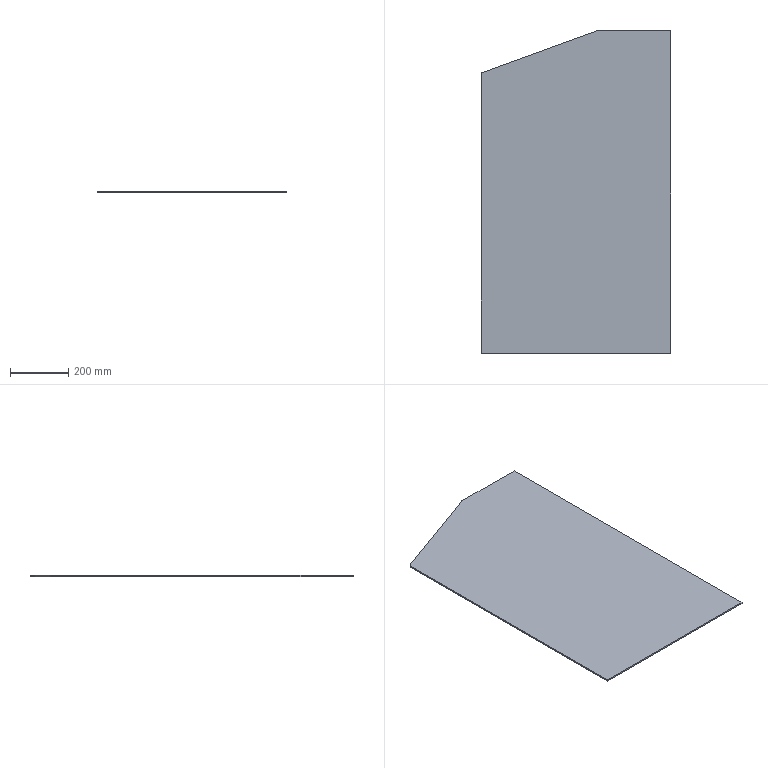Part | SolidWorks | features Extrusion 1, Fillet 1 | 1 solid | 9 faces | box 651 x 1106 x 5 mm | volume 3454699 mm3 | plane 7 | cylinder 2 | commonest cylinder face diameters 12 x2
STEP:
#1=CARTESIAN_POINT('',(-651.,0.,0.));
#2=VERTEX_POINT('',#1);
#3=CARTESIAN_POINT('',(0.,0.,0.));
#4=VERTEX_POINT('',#3);
#5=CARTESIAN_POINT('',(-651.,0.,0.));
#6=DIRECTION('',(1.,0.,0.));
#7=VECTOR('',#6,1000.);
#8=LINE('',#5,#7);
#9=EDGE_CURVE('',#2,#4,#8,.T.);
#10=ORIENTED_EDGE('',*,*,#9,.T.);
#11=CARTESIAN_POINT('',(0.,0.,5.));
#12=VERTEX_POINT('',#11);
#13=CARTESIAN_POINT('',(0.,0.,5.));
#14=DIRECTION('',(0.,0.,-1.));
#15=VECTOR('',#14,1000.);
#16=LINE('',#13,#15);
#17=EDGE_CURVE('',#12,#4,#16,.T.);
#18=ORIENTED_EDGE('',*,*,#17,.F.);
#19=CARTESIAN_POINT('',(-651.,0.,5.));
#20=VERTEX_POINT('',#19);
#21=CARTESIAN_POINT('',(-651.,0.,5.));
#22=DIRECTION('',(1.,0.,0.));
#23=VECTOR('',#22,1000.);
#24=LINE('',#21,#23);
#25=EDGE_CURVE('',#20,#12,#24,.T.);
#26=ORIENTED_EDGE('',*,*,#25,.F.);
#27=CARTESIAN_POINT('',(-651.,0.,5.));
#28=DIRECTION('',(0.,0.,-1.));
#29=VECTOR('',#28,1000.);
#30=LINE('',#27,#29);
#31=EDGE_CURVE('',#20,#2,#30,.T.);
#32=ORIENTED_EDGE('',*,*,#31,.T.);
#33=EDGE_LOOP('',(#10,#18,#26,#32));
#34=FACE_OUTER_BOUND('',#33,.T.);
#35=CARTESIAN_POINT('',(-651.,0.,5.));
#36=DIRECTION('',(0.,1.,0.));
#37=DIRECTION('',(0.,0.,1.));
#38=AXIS2_PLACEMENT_3D('',#35,#36,#37);
#39=PLANE('',#38);
#40=ADVANCED_FACE('',(#34),#39,.F.);
#41=CARTESIAN_POINT('',(0.,1105.5,0.));
#42=VERTEX_POINT('',#41);
#43=CARTESIAN_POINT('',(0.,0.,0.));
#44=DIRECTION('',(0.,1.,0.));
#45=VECTOR('',#44,1000.);
#46=LINE('',#43,#45);
#47=EDGE_CURVE('',#4,#42,#46,.T.);
#48=ORIENTED_EDGE('',*,*,#47,.T.);
#49=CARTESIAN_POINT('',(0.,1105.5,5.));
#50=VERTEX_POINT('',#49);
#51=CARTESIAN_POINT('',(0.,1105.5,5.));
#52=DIRECTION('',(0.,0.,-1.));
#53=VECTOR('',#52,1000.);
#54=LINE('',#51,#53);
#55=EDGE_CURVE('',#50,#42,#54,.T.);
#56=ORIENTED_EDGE('',*,*,#55,.F.);
#57=CARTESIAN_POINT('',(0.,0.,5.));
#58=DIRECTION('',(0.,1.,0.));
#59=VECTOR('',#58,1000.);
#60=LINE('',#57,#59);
#61=EDGE_CURVE('',#12,#50,#60,.T.);
#62=ORIENTED_EDGE('',*,*,#61,.F.);
#63=ORIENTED_EDGE('',*,*,#17,.T.);
#64=EDGE_LOOP('',(#48,#56,#62,#63));
#65=FACE_OUTER_BOUND('',#64,.T.);
#66=CARTESIAN_POINT('',(0.,0.,5.));
#67=DIRECTION('',(-1.,0.,0.));
#68=DIRECTION('',(0.,0.,1.));
#69=AXIS2_PLACEMENT_3D('',#66,#67,#68);
#70=PLANE('',#69);
#71=ADVANCED_FACE('',(#65),#70,.F.);
#72=CARTESIAN_POINT('',(-252.562,1105.5,0.));
#73=VERTEX_POINT('',#72);
#74=CARTESIAN_POINT('',(0.,1105.5,0.));
#75=DIRECTION('',(-1.,0.,0.));
#76=VECTOR('',#75,1000.);
#77=LINE('',#74,#76);
#78=EDGE_CURVE('',#42,#73,#77,.T.);
#79=ORIENTED_EDGE('',*,*,#78,.T.);
#80=CARTESIAN_POINT('',(-252.562,1105.5,5.));
#81=VERTEX_POINT('',#80);
#82=CARTESIAN_POINT('',(-252.562,1105.5,5.));
#83=DIRECTION('',(0.,0.,1.));
#84=VECTOR('',#83,1000.);
#85=LINE('',#82,#84);
#86=EDGE_CURVE('',#73,#81,#85,.T.);
#87=ORIENTED_EDGE('',*,*,#86,.T.);
#88=CARTESIAN_POINT('',(0.,1105.5,5.));
#89=DIRECTION('',(-1.,0.,0.));
#90=VECTOR('',#89,1000.);
#91=LINE('',#88,#90);
#92=EDGE_CURVE('',#50,#81,#91,.T.);
#93=ORIENTED_EDGE('',*,*,#92,.F.);
#94=ORIENTED_EDGE('',*,*,#55,.T.);
#95=EDGE_LOOP('',(#79,#87,#93,#94));
#96=FACE_OUTER_BOUND('',#95,.T.);
#97=CARTESIAN_POINT('',(0.,1105.5,5.));
#98=DIRECTION('',(0.,-1.,0.));
#99=DIRECTION('',(0.,0.,-1.));
#100=AXIS2_PLACEMENT_3D('',#97,#98,#99);
#101=PLANE('',#100);
#102=ADVANCED_FACE('',(#96),#101,.F.);
#103=CARTESIAN_POINT('',(-254.614,1105.138,5.));
#104=VERTEX_POINT('',#103);
#105=CARTESIAN_POINT('',(-647.052,962.302,5.));
#106=VERTEX_POINT('',#105);
#107=CARTESIAN_POINT('',(-253.62,1105.5,5.));
#108=DIRECTION('',(-0.9397,-0.342,0.));
#109=VECTOR('',#108,1000.);
#110=LINE('',#107,#109);
#111=EDGE_CURVE('',#104,#106,#110,.T.);
#112=ORIENTED_EDGE('',*,*,#111,.F.);
#113=CARTESIAN_POINT('',(-254.614,1105.138,0.));
#114=VERTEX_POINT('',#113);
#115=CARTESIAN_POINT('',(-254.614,1105.138,5.));
#116=DIRECTION('',(0.,0.,-1.));
#117=VECTOR('',#116,1000.);
#118=LINE('',#115,#117);
#119=EDGE_CURVE('',#104,#114,#118,.T.);
#120=ORIENTED_EDGE('',*,*,#119,.T.);
#121=CARTESIAN_POINT('',(-647.052,962.302,0.));
#122=VERTEX_POINT('',#121);
#123=CARTESIAN_POINT('',(-253.62,1105.5,0.));
#124=DIRECTION('',(-0.9397,-0.342,0.));
#125=VECTOR('',#124,1000.);
#126=LINE('',#123,#125);
#127=EDGE_CURVE('',#114,#122,#126,.T.);
#128=ORIENTED_EDGE('',*,*,#127,.T.);
#129=CARTESIAN_POINT('',(-647.052,962.302,5.));
#130=DIRECTION('',(0.,0.,1.));
#131=VECTOR('',#130,1000.);
#132=LINE('',#129,#131);
#133=EDGE_CURVE('',#122,#106,#132,.T.);
#134=ORIENTED_EDGE('',*,*,#133,.T.);
#135=EDGE_LOOP('',(#112,#120,#128,#134));
#136=FACE_OUTER_BOUND('',#135,.T.);
#137=CARTESIAN_POINT('',(-253.62,1105.5,5.));
#138=DIRECTION('',(0.342,-0.9397,0.));
#139=DIRECTION('',(0.9397,0.342,0.));
#140=AXIS2_PLACEMENT_3D('',#137,#138,#139);
#141=PLANE('',#140);
#142=ADVANCED_FACE('',(#136),#141,.F.);
#143=CARTESIAN_POINT('',(-651.,956.664,5.));
#144=VERTEX_POINT('',#143);
#145=CARTESIAN_POINT('',(-651.,960.866,5.));
#146=DIRECTION('',(0.,-1.,0.));
#147=VECTOR('',#146,1000.);
#148=LINE('',#145,#147);
#149=EDGE_CURVE('',#144,#20,#148,.T.);
#150=ORIENTED_EDGE('',*,*,#149,.F.);
#151=CARTESIAN_POINT('',(-651.,956.664,0.));
#152=VERTEX_POINT('',#151);
#153=CARTESIAN_POINT('',(-651.,956.664,5.));
#154=DIRECTION('',(0.,0.,-1.));
#155=VECTOR('',#154,1000.);
#156=LINE('',#153,#155);
#157=EDGE_CURVE('',#144,#152,#156,.T.);
#158=ORIENTED_EDGE('',*,*,#157,.T.);
#159=CARTESIAN_POINT('',(-651.,960.866,0.));
#160=DIRECTION('',(0.,-1.,0.));
#161=VECTOR('',#160,1000.);
#162=LINE('',#159,#161);
#163=EDGE_CURVE('',#152,#2,#162,.T.);
#164=ORIENTED_EDGE('',*,*,#163,.T.);
#165=ORIENTED_EDGE('',*,*,#31,.F.);
#166=EDGE_LOOP('',(#150,#158,#164,#165));
#167=FACE_OUTER_BOUND('',#166,.T.);
#168=CARTESIAN_POINT('',(-651.,960.866,5.));
#169=DIRECTION('',(1.,0.,0.));
#170=DIRECTION('',(0.,1.,0.));
#171=AXIS2_PLACEMENT_3D('',#168,#169,#170);
#172=PLANE('',#171);
#173=ADVANCED_FACE('',(#167),#172,.F.);
#174=ORIENTED_EDGE('',*,*,#92,.T.);
#175=CARTESIAN_POINT('',(-252.562,1099.5,5.));
#176=DIRECTION('',(0.,0.,1.));
#177=DIRECTION('',(1.,0.,0.));
#178=AXIS2_PLACEMENT_3D('',#175,#176,#177);
#179=CIRCLE('',#178,6.);
#180=EDGE_CURVE('',#81,#104,#179,.T.);
#181=ORIENTED_EDGE('',*,*,#180,.T.);
#182=ORIENTED_EDGE('',*,*,#111,.T.);
#183=CARTESIAN_POINT('',(-645.,956.664,5.));
#184=DIRECTION('',(0.,0.,1.));
#185=DIRECTION('',(1.,0.,0.));
#186=AXIS2_PLACEMENT_3D('',#183,#184,#185);
#187=CIRCLE('',#186,6.);
#188=EDGE_CURVE('',#106,#144,#187,.T.);
#189=ORIENTED_EDGE('',*,*,#188,.T.);
#190=ORIENTED_EDGE('',*,*,#149,.T.);
#191=ORIENTED_EDGE('',*,*,#25,.T.);
#192=ORIENTED_EDGE('',*,*,#61,.T.);
#193=EDGE_LOOP('',(#174,#181,#182,#189,#190,#191,#192));
#194=FACE_OUTER_BOUND('',#193,.T.);
#195=CARTESIAN_POINT('',(0.,0.,5.));
#196=DIRECTION('',(0.,0.,1.));
#197=DIRECTION('',(1.,0.,0.));
#198=AXIS2_PLACEMENT_3D('',#195,#196,#197);
#199=PLANE('',#198);
#200=ADVANCED_FACE('',(#194),#199,.T.);
#201=ORIENTED_EDGE('',*,*,#127,.F.);
#202=CARTESIAN_POINT('',(-252.562,1099.5,0.));
#203=DIRECTION('',(0.,0.,-1.));
#204=DIRECTION('',(1.,0.,0.));
#205=AXIS2_PLACEMENT_3D('',#202,#203,#204);
#206=CIRCLE('',#205,6.);
#207=EDGE_CURVE('',#114,#73,#206,.T.);
#208=ORIENTED_EDGE('',*,*,#207,.T.);
#209=ORIENTED_EDGE('',*,*,#78,.F.);
#210=ORIENTED_EDGE('',*,*,#47,.F.);
#211=ORIENTED_EDGE('',*,*,#9,.F.);
#212=ORIENTED_EDGE('',*,*,#163,.F.);
#213=CARTESIAN_POINT('',(-645.,956.664,0.));
#214=DIRECTION('',(0.,0.,-1.));
#215=DIRECTION('',(1.,0.,0.));
#216=AXIS2_PLACEMENT_3D('',#213,#214,#215);
#217=CIRCLE('',#216,6.);
#218=EDGE_CURVE('',#152,#122,#217,.T.);
#219=ORIENTED_EDGE('',*,*,#218,.T.);
#220=EDGE_LOOP('',(#201,#208,#209,#210,#211,#212,#219));
#221=FACE_OUTER_BOUND('',#220,.T.);
#222=CARTESIAN_POINT('',(0.,0.,0.));
#223=DIRECTION('',(0.,0.,1.));
#224=DIRECTION('',(1.,0.,0.));
#225=AXIS2_PLACEMENT_3D('',#222,#223,#224);
#226=PLANE('',#225);
#227=ADVANCED_FACE('',(#221),#226,.F.);
#228=ORIENTED_EDGE('',*,*,#180,.F.);
#229=ORIENTED_EDGE('',*,*,#86,.F.);
#230=ORIENTED_EDGE('',*,*,#207,.F.);
#231=ORIENTED_EDGE('',*,*,#119,.F.);
#232=EDGE_LOOP('',(#228,#229,#230,#231));
#233=FACE_OUTER_BOUND('',#232,.T.);
#234=CARTESIAN_POINT('',(-252.562,1099.5,5.));
#235=DIRECTION('',(0.,0.,-1.));
#236=DIRECTION('',(-1.,0.,0.));
#237=AXIS2_PLACEMENT_3D('',#234,#235,#236);
#238=CYLINDRICAL_SURFACE('',#237,6.);
#239=ADVANCED_FACE('',(#233),#238,.T.);
#240=ORIENTED_EDGE('',*,*,#188,.F.);
#241=ORIENTED_EDGE('',*,*,#133,.F.);
#242=ORIENTED_EDGE('',*,*,#218,.F.);
#243=ORIENTED_EDGE('',*,*,#157,.F.);
#244=EDGE_LOOP('',(#240,#241,#242,#243));
#245=FACE_OUTER_BOUND('',#244,.T.);
#246=CARTESIAN_POINT('',(-645.,956.664,5.));
#247=DIRECTION('',(0.,0.,-1.));
#248=DIRECTION('',(-1.,0.,0.));
#249=AXIS2_PLACEMENT_3D('',#246,#247,#248);
#250=CYLINDRICAL_SURFACE('',#249,6.);
#251=ADVANCED_FACE('',(#245),#250,.T.);
#252=CLOSED_SHELL('',(#40,#71,#102,#142,#173,#200,#227,#239,#251));
#253=MANIFOLD_SOLID_BREP('',#252);
#254=CARTESIAN_POINT('',(0.,0.,0.));
#255=DIRECTION('',(0.,0.,1.));
#256=DIRECTION('',(1.,0.,0.));
#257=AXIS2_PLACEMENT_3D('',#254,#255,#256);
#258=(LENGTH_UNIT()NAMED_UNIT(*)SI_UNIT(.MILLI.,.METRE.));
#259=UNCERTAINTY_MEASURE_WITH_UNIT(LENGTH_MEASURE(0.00001),#258,'','');
#260=(NAMED_UNIT(*)PLANE_ANGLE_UNIT()SI_UNIT($,.RADIAN.));
#261=(NAMED_UNIT(*)SI_UNIT($,.STERADIAN.)SOLID_ANGLE_UNIT());
#262=(GEOMETRIC_REPRESENTATION_CONTEXT(3)GLOBAL_UNCERTAINTY_ASSIGNED_CONTEXT((#259))GLOBAL_UNIT_ASSIGNED_CONTEXT((#258,#260,#261))REPRESENTATION_CONTEXT('',''));
#263=ADVANCED_BREP_SHAPE_REPRESENTATION('',(#253,#257),#262);